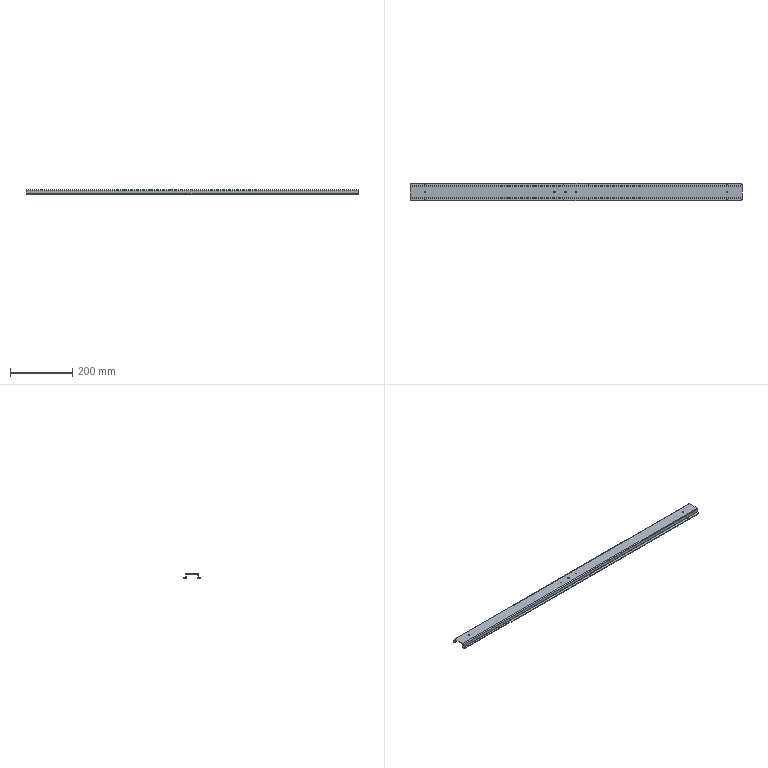Part | SolidWorks | features EdgeFlange 2, ICE 2, Cut 1, Fillet 1, FlatPattern 1, HoleWzd 1, MoveFace 1, SMBaseFlange 1, SheetMetal 1 | 1 solid | 68 faces | box 1065 x 56 x 15 mm | volume 167971 mm3 | cylinder 38 | plane 30 | commonest cylinder face diameters 4.2 x10 3 x8 4 x8 1.473 x4 5.473 x4 10 x4